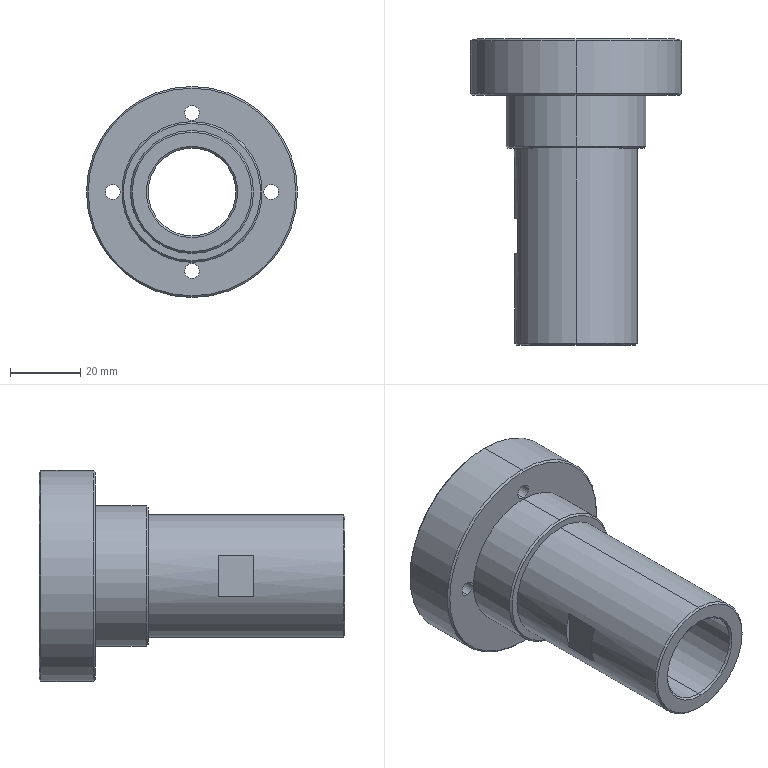Part | SolidWorks | features BaseBody 1 | 1 solid | 33 faces | box 60 x 87 x 60 mm | volume 74210 mm3 | cylinder 16 | cone 10 | plane 7 | commonest cylinder face diameters 4.2 x8 25 x2 35 x2 40 x2 60 x2
STEP:
#1=CARTESIAN_POINT('',(0.,-70.5,12.5));
#2=VERTEX_POINT('',#1);
#3=CARTESIAN_POINT('',(0.,-71.,13.));
#4=VERTEX_POINT('',#3);
#5=CARTESIAN_POINT('',(0.,-71.,13.));
#6=DIRECTION('',(0.,-0.7071,0.7071));
#7=VECTOR('',#6,1000.);
#8=LINE('',#5,#7);
#9=EDGE_CURVE('',#2,#4,#8,.T.);
#10=ORIENTED_EDGE('',*,*,#9,.F.);
#11=CARTESIAN_POINT('',(0.,-70.5,-12.5));
#12=VERTEX_POINT('',#11);
#13=CARTESIAN_POINT('',(0.,-70.5,0.));
#14=DIRECTION('',(0.,-1.,0.));
#15=DIRECTION('',(0.,0.,-1.));
#16=AXIS2_PLACEMENT_3D('',#13,#14,#15);
#17=CIRCLE('',#16,12.5);
#18=EDGE_CURVE('',#12,#2,#17,.T.);
#19=ORIENTED_EDGE('',*,*,#18,.F.);
#20=CARTESIAN_POINT('',(0.,-71.,-13.));
#21=VERTEX_POINT('',#20);
#22=CARTESIAN_POINT('',(0.,-71.,-13.));
#23=DIRECTION('',(0.,-0.7071,-0.7071));
#24=VECTOR('',#23,1000.);
#25=LINE('',#22,#24);
#26=EDGE_CURVE('',#12,#21,#25,.T.);
#27=ORIENTED_EDGE('',*,*,#26,.T.);
#28=CARTESIAN_POINT('',(0.,-71.,0.));
#29=DIRECTION('',(0.,1.,0.));
#30=DIRECTION('',(0.,0.,-1.));
#31=AXIS2_PLACEMENT_3D('',#28,#29,#30);
#32=CIRCLE('',#31,13.);
#33=EDGE_CURVE('',#4,#21,#32,.T.);
#34=ORIENTED_EDGE('',*,*,#33,.F.);
#35=EDGE_LOOP('',(#10,#19,#27,#34));
#36=FACE_OUTER_BOUND('',#35,.T.);
#37=CARTESIAN_POINT('',(0.,-71.,0.));
#38=DIRECTION('',(0.,-1.,0.));
#39=DIRECTION('',(0.,0.,-1.));
#40=AXIS2_PLACEMENT_3D('',#37,#38,#39);
#41=CONICAL_SURFACE('',#40,13.,0.7854);
#42=ADVANCED_FACE('',(#36),#41,.F.);
#43=CARTESIAN_POINT('',(-16.5,-45.,-5.831));
#44=VERTEX_POINT('',#43);
#45=CARTESIAN_POINT('',(-16.5,-45.,5.831));
#46=VERTEX_POINT('',#45);
#47=CARTESIAN_POINT('',(-16.5,-45.,-15.));
#48=DIRECTION('',(0.,0.,1.));
#49=VECTOR('',#48,1000.);
#50=LINE('',#47,#49);
#51=EDGE_CURVE('',#44,#46,#50,.T.);
#52=ORIENTED_EDGE('',*,*,#51,.F.);
#53=CARTESIAN_POINT('',(0.,-45.,0.));
#54=DIRECTION('',(0.,-1.,0.));
#55=DIRECTION('',(0.,0.,-1.));
#56=AXIS2_PLACEMENT_3D('',#53,#54,#55);
#57=CIRCLE('',#56,17.5);
#58=EDGE_CURVE('',#46,#44,#57,.T.);
#59=ORIENTED_EDGE('',*,*,#58,.F.);
#60=EDGE_LOOP('',(#52,#59));
#61=FACE_OUTER_BOUND('',#60,.T.);
#62=CARTESIAN_POINT('',(-17.5,-45.,-15.));
#63=DIRECTION('',(0.,-1.,0.));
#64=DIRECTION('',(0.,0.,-1.));
#65=AXIS2_PLACEMENT_3D('',#62,#63,#64);
#66=PLANE('',#65);
#67=ADVANCED_FACE('',(#61),#66,.F.);
#68=ORIENTED_EDGE('',*,*,#51,.T.);
#69=CARTESIAN_POINT('',(-16.5,-35.,5.831));
#70=VERTEX_POINT('',#69);
#71=CARTESIAN_POINT('',(-16.5,-71.,5.831));
#72=DIRECTION('',(0.,-1.,0.));
#73=VECTOR('',#72,1000.);
#74=LINE('',#71,#73);
#75=EDGE_CURVE('',#70,#46,#74,.T.);
#76=ORIENTED_EDGE('',*,*,#75,.F.);
#77=CARTESIAN_POINT('',(-16.5,-35.,-5.831));
#78=VERTEX_POINT('',#77);
#79=CARTESIAN_POINT('',(-16.5,-35.,-15.));
#80=DIRECTION('',(0.,0.,1.));
#81=VECTOR('',#80,1000.);
#82=LINE('',#79,#81);
#83=EDGE_CURVE('',#78,#70,#82,.T.);
#84=ORIENTED_EDGE('',*,*,#83,.F.);
#85=CARTESIAN_POINT('',(-16.5,-71.,-5.831));
#86=DIRECTION('',(0.,1.,0.));
#87=VECTOR('',#86,1000.);
#88=LINE('',#85,#87);
#89=EDGE_CURVE('',#44,#78,#88,.T.);
#90=ORIENTED_EDGE('',*,*,#89,.F.);
#91=EDGE_LOOP('',(#68,#76,#84,#90));
#92=FACE_OUTER_BOUND('',#91,.T.);
#93=CARTESIAN_POINT('',(-16.5,-45.,-15.));
#94=DIRECTION('',(1.,0.,0.));
#95=DIRECTION('',(0.,1.,0.));
#96=AXIS2_PLACEMENT_3D('',#93,#94,#95);
#97=PLANE('',#96);
#98=ADVANCED_FACE('',(#92),#97,.F.);
#99=ORIENTED_EDGE('',*,*,#83,.T.);
#100=CARTESIAN_POINT('',(0.,-35.,0.));
#101=DIRECTION('',(0.,1.,0.));
#102=DIRECTION('',(0.,0.,1.));
#103=AXIS2_PLACEMENT_3D('',#100,#101,#102);
#104=CIRCLE('',#103,17.5);
#105=EDGE_CURVE('',#78,#70,#104,.T.);
#106=ORIENTED_EDGE('',*,*,#105,.F.);
#107=EDGE_LOOP('',(#99,#106));
#108=FACE_OUTER_BOUND('',#107,.T.);
#109=CARTESIAN_POINT('',(-17.5,-35.,-15.));
#110=DIRECTION('',(0.,1.,0.));
#111=DIRECTION('',(1.,0.,0.));
#112=AXIS2_PLACEMENT_3D('',#109,#110,#111);
#113=PLANE('',#112);
#114=ADVANCED_FACE('',(#108),#113,.F.);
#115=CARTESIAN_POINT('',(0.,16.,-12.5));
#116=VERTEX_POINT('',#115);
#117=CARTESIAN_POINT('',(0.,-106.355,-12.5));
#118=DIRECTION('',(0.,1.,0.));
#119=VECTOR('',#118,1000.);
#120=LINE('',#117,#119);
#121=EDGE_CURVE('',#12,#116,#120,.T.);
#122=ORIENTED_EDGE('',*,*,#121,.F.);
#123=ORIENTED_EDGE('',*,*,#18,.T.);
#124=CARTESIAN_POINT('',(0.,16.,12.5));
#125=VERTEX_POINT('',#124);
#126=CARTESIAN_POINT('',(0.,-106.355,12.5));
#127=DIRECTION('',(0.,1.,0.));
#128=VECTOR('',#127,1000.);
#129=LINE('',#126,#128);
#130=EDGE_CURVE('',#2,#125,#129,.T.);
#131=ORIENTED_EDGE('',*,*,#130,.T.);
#132=CARTESIAN_POINT('',(0.,16.,0.));
#133=DIRECTION('',(0.,1.,0.));
#134=DIRECTION('',(0.,0.,1.));
#135=AXIS2_PLACEMENT_3D('',#132,#133,#134);
#136=CIRCLE('',#135,12.5);
#137=EDGE_CURVE('',#125,#116,#136,.T.);
#138=ORIENTED_EDGE('',*,*,#137,.T.);
#139=EDGE_LOOP('',(#122,#123,#131,#138));
#140=FACE_OUTER_BOUND('',#139,.T.);
#141=CARTESIAN_POINT('',(0.,-106.355,0.));
#142=DIRECTION('',(0.,1.,0.));
#143=DIRECTION('',(0.,0.,1.));
#144=AXIS2_PLACEMENT_3D('',#141,#142,#143);
#145=CYLINDRICAL_SURFACE('',#144,12.5);
#146=ADVANCED_FACE('',(#140),#145,.F.);
#147=CARTESIAN_POINT('',(0.,0.,20.4));
#148=VERTEX_POINT('',#147);
#149=CARTESIAN_POINT('',(0.,16.,20.4));
#150=VERTEX_POINT('',#149);
#151=CARTESIAN_POINT('',(0.,16.,20.4));
#152=DIRECTION('',(0.,1.,0.));
#153=VECTOR('',#152,1000.);
#154=LINE('',#151,#153);
#155=EDGE_CURVE('',#148,#150,#154,.T.);
#156=ORIENTED_EDGE('',*,*,#155,.F.);
#157=CARTESIAN_POINT('',(0.,0.,24.6));
#158=VERTEX_POINT('',#157);
#159=CARTESIAN_POINT('',(0.,0.,22.5));
#160=DIRECTION('',(0.,1.,0.));
#161=DIRECTION('',(0.,0.,1.));
#162=AXIS2_PLACEMENT_3D('',#159,#160,#161);
#163=CIRCLE('',#162,2.1);
#164=EDGE_CURVE('',#158,#148,#163,.T.);
#165=ORIENTED_EDGE('',*,*,#164,.F.);
#166=CARTESIAN_POINT('',(0.,16.,24.6));
#167=VERTEX_POINT('',#166);
#168=CARTESIAN_POINT('',(0.,16.,24.6));
#169=DIRECTION('',(0.,1.,0.));
#170=VECTOR('',#169,1000.);
#171=LINE('',#168,#170);
#172=EDGE_CURVE('',#158,#167,#171,.T.);
#173=ORIENTED_EDGE('',*,*,#172,.T.);
#174=CARTESIAN_POINT('',(0.,16.,22.5));
#175=DIRECTION('',(0.,1.,0.));
#176=DIRECTION('',(0.,0.,1.));
#177=AXIS2_PLACEMENT_3D('',#174,#175,#176);
#178=CIRCLE('',#177,2.1);
#179=EDGE_CURVE('',#167,#150,#178,.T.);
#180=ORIENTED_EDGE('',*,*,#179,.T.);
#181=EDGE_LOOP('',(#156,#165,#173,#180));
#182=FACE_OUTER_BOUND('',#181,.T.);
#183=CARTESIAN_POINT('',(0.,16.,22.5));
#184=DIRECTION('',(0.,1.,0.));
#185=DIRECTION('',(0.,0.,1.));
#186=AXIS2_PLACEMENT_3D('',#183,#184,#185);
#187=CYLINDRICAL_SURFACE('',#186,2.1);
#188=ADVANCED_FACE('',(#182),#187,.F.);
#189=CARTESIAN_POINT('',(0.,0.,-24.6));
#190=VERTEX_POINT('',#189);
#191=CARTESIAN_POINT('',(0.,16.,-24.6));
#192=VERTEX_POINT('',#191);
#193=CARTESIAN_POINT('',(0.,16.,-24.6));
#194=DIRECTION('',(0.,1.,0.));
#195=VECTOR('',#194,1000.);
#196=LINE('',#193,#195);
#197=EDGE_CURVE('',#190,#192,#196,.T.);
#198=ORIENTED_EDGE('',*,*,#197,.F.);
#199=CARTESIAN_POINT('',(0.,0.,-20.4));
#200=VERTEX_POINT('',#199);
#201=CARTESIAN_POINT('',(0.,0.,-22.5));
#202=DIRECTION('',(0.,1.,0.));
#203=DIRECTION('',(0.,0.,1.));
#204=AXIS2_PLACEMENT_3D('',#201,#202,#203);
#205=CIRCLE('',#204,2.1);
#206=EDGE_CURVE('',#200,#190,#205,.T.);
#207=ORIENTED_EDGE('',*,*,#206,.F.);
#208=CARTESIAN_POINT('',(0.,16.,-20.4));
#209=VERTEX_POINT('',#208);
#210=CARTESIAN_POINT('',(0.,16.,-20.4));
#211=DIRECTION('',(0.,1.,0.));
#212=VECTOR('',#211,1000.);
#213=LINE('',#210,#212);
#214=EDGE_CURVE('',#200,#209,#213,.T.);
#215=ORIENTED_EDGE('',*,*,#214,.T.);
#216=CARTESIAN_POINT('',(0.,16.,-22.5));
#217=DIRECTION('',(0.,1.,0.));
#218=DIRECTION('',(0.,0.,1.));
#219=AXIS2_PLACEMENT_3D('',#216,#217,#218);
#220=CIRCLE('',#219,2.1);
#221=EDGE_CURVE('',#209,#192,#220,.T.);
#222=ORIENTED_EDGE('',*,*,#221,.T.);
#223=EDGE_LOOP('',(#198,#207,#215,#222));
#224=FACE_OUTER_BOUND('',#223,.T.);
#225=CARTESIAN_POINT('',(0.,16.,-22.5));
#226=DIRECTION('',(0.,1.,0.));
#227=DIRECTION('',(0.,0.,1.));
#228=AXIS2_PLACEMENT_3D('',#225,#226,#227);
#229=CYLINDRICAL_SURFACE('',#228,2.1);
#230=ADVANCED_FACE('',(#224),#229,.F.);
#231=CARTESIAN_POINT('',(22.5,0.,-2.1));
#232=VERTEX_POINT('',#231);
#233=CARTESIAN_POINT('',(22.5,16.,-2.1));
#234=VERTEX_POINT('',#233);
#235=CARTESIAN_POINT('',(22.5,16.,-2.1));
#236=DIRECTION('',(0.,1.,0.));
#237=VECTOR('',#236,1000.);
#238=LINE('',#235,#237);
#239=EDGE_CURVE('',#232,#234,#238,.T.);
#240=ORIENTED_EDGE('',*,*,#239,.F.);
#241=CARTESIAN_POINT('',(22.5,0.,2.1));
#242=VERTEX_POINT('',#241);
#243=CARTESIAN_POINT('',(22.5,0.,0.));
#244=DIRECTION('',(0.,1.,0.));
#245=DIRECTION('',(0.,0.,1.));
#246=AXIS2_PLACEMENT_3D('',#243,#244,#245);
#247=CIRCLE('',#246,2.1);
#248=EDGE_CURVE('',#242,#232,#247,.T.);
#249=ORIENTED_EDGE('',*,*,#248,.F.);
#250=CARTESIAN_POINT('',(22.5,16.,2.1));
#251=VERTEX_POINT('',#250);
#252=CARTESIAN_POINT('',(22.5,16.,2.1));
#253=DIRECTION('',(0.,1.,0.));
#254=VECTOR('',#253,1000.);
#255=LINE('',#252,#254);
#256=EDGE_CURVE('',#242,#251,#255,.T.);
#257=ORIENTED_EDGE('',*,*,#256,.T.);
#258=CARTESIAN_POINT('',(22.5,16.,0.));
#259=DIRECTION('',(0.,1.,0.));
#260=DIRECTION('',(0.,0.,1.));
#261=AXIS2_PLACEMENT_3D('',#258,#259,#260);
#262=CIRCLE('',#261,2.1);
#263=EDGE_CURVE('',#251,#234,#262,.T.);
#264=ORIENTED_EDGE('',*,*,#263,.T.);
#265=EDGE_LOOP('',(#240,#249,#257,#264));
#266=FACE_OUTER_BOUND('',#265,.T.);
#267=CARTESIAN_POINT('',(22.5,16.,0.));
#268=DIRECTION('',(0.,1.,0.));
#269=DIRECTION('',(0.,0.,1.));
#270=AXIS2_PLACEMENT_3D('',#267,#268,#269);
#271=CYLINDRICAL_SURFACE('',#270,2.1);
#272=ADVANCED_FACE('',(#266),#271,.F.);
#273=CARTESIAN_POINT('',(-22.5,0.,-2.1));
#274=VERTEX_POINT('',#273);
#275=CARTESIAN_POINT('',(-22.5,16.,-2.1));
#276=VERTEX_POINT('',#275);
#277=CARTESIAN_POINT('',(-22.5,16.,-2.1));
#278=DIRECTION('',(0.,1.,0.));
#279=VECTOR('',#278,1000.);
#280=LINE('',#277,#279);
#281=EDGE_CURVE('',#274,#276,#280,.T.);
#282=ORIENTED_EDGE('',*,*,#281,.F.);
#283=CARTESIAN_POINT('',(-22.5,0.,2.1));
#284=VERTEX_POINT('',#283);
#285=CARTESIAN_POINT('',(-22.5,0.,0.));
#286=DIRECTION('',(0.,1.,0.));
#287=DIRECTION('',(0.,0.,1.));
#288=AXIS2_PLACEMENT_3D('',#285,#286,#287);
#289=CIRCLE('',#288,2.1);
#290=EDGE_CURVE('',#284,#274,#289,.T.);
#291=ORIENTED_EDGE('',*,*,#290,.F.);
#292=CARTESIAN_POINT('',(-22.5,16.,2.1));
#293=VERTEX_POINT('',#292);
#294=CARTESIAN_POINT('',(-22.5,16.,2.1));
#295=DIRECTION('',(0.,1.,0.));
#296=VECTOR('',#295,1000.);
#297=LINE('',#294,#296);
#298=EDGE_CURVE('',#284,#293,#297,.T.);
#299=ORIENTED_EDGE('',*,*,#298,.T.);
#300=CARTESIAN_POINT('',(-22.5,16.,0.));
#301=DIRECTION('',(0.,1.,0.));
#302=DIRECTION('',(0.,0.,1.));
#303=AXIS2_PLACEMENT_3D('',#300,#301,#302);
#304=CIRCLE('',#303,2.1);
#305=EDGE_CURVE('',#293,#276,#304,.T.);
#306=ORIENTED_EDGE('',*,*,#305,.T.);
#307=EDGE_LOOP('',(#282,#291,#299,#306));
#308=FACE_OUTER_BOUND('',#307,.T.);
#309=CARTESIAN_POINT('',(-22.5,16.,0.));
#310=DIRECTION('',(0.,1.,0.));
#311=DIRECTION('',(0.,0.,1.));
#312=AXIS2_PLACEMENT_3D('',#309,#310,#311);
#313=CYLINDRICAL_SURFACE('',#312,2.1);
#314=ADVANCED_FACE('',(#308),#313,.F.);
#315=CARTESIAN_POINT('',(0.,16.,29.5));
#316=VERTEX_POINT('',#315);
#317=CARTESIAN_POINT('',(0.,15.5,30.));
#318=VERTEX_POINT('',#317);
#319=CARTESIAN_POINT('',(0.,16.,29.5));
#320=DIRECTION('',(0.,-0.7071,0.7071));
#321=VECTOR('',#320,1000.);
#322=LINE('',#319,#321);
#323=EDGE_CURVE('',#316,#318,#322,.T.);
#324=ORIENTED_EDGE('',*,*,#323,.F.);
#325=CARTESIAN_POINT('',(0.,16.,-29.5));
#326=VERTEX_POINT('',#325);
#327=CARTESIAN_POINT('',(0.,16.,0.));
#328=DIRECTION('',(0.,1.,0.));
#329=DIRECTION('',(0.,0.,1.));
#330=AXIS2_PLACEMENT_3D('',#327,#328,#329);
#331=CIRCLE('',#330,29.5);
#332=EDGE_CURVE('',#326,#316,#331,.T.);
#333=ORIENTED_EDGE('',*,*,#332,.F.);
#334=CARTESIAN_POINT('',(0.,15.5,-30.));
#335=VERTEX_POINT('',#334);
#336=CARTESIAN_POINT('',(0.,16.,-29.5));
#337=DIRECTION('',(0.,-0.7071,-0.7071));
#338=VECTOR('',#337,1000.);
#339=LINE('',#336,#338);
#340=EDGE_CURVE('',#326,#335,#339,.T.);
#341=ORIENTED_EDGE('',*,*,#340,.T.);
#342=CARTESIAN_POINT('',(0.,15.5,0.));
#343=DIRECTION('',(0.,-1.,0.));
#344=DIRECTION('',(0.,0.,1.));
#345=AXIS2_PLACEMENT_3D('',#342,#343,#344);
#346=CIRCLE('',#345,30.);
#347=EDGE_CURVE('',#318,#335,#346,.T.);
#348=ORIENTED_EDGE('',*,*,#347,.F.);
#349=EDGE_LOOP('',(#324,#333,#341,#348));
#350=FACE_OUTER_BOUND('',#349,.T.);
#351=CARTESIAN_POINT('',(0.,16.,0.));
#352=DIRECTION('',(0.,-1.,0.));
#353=DIRECTION('',(0.,0.,-1.));
#354=AXIS2_PLACEMENT_3D('',#351,#352,#353);
#355=CONICAL_SURFACE('',#354,29.5,0.7854);
#356=ADVANCED_FACE('',(#350),#355,.T.);
#357=CARTESIAN_POINT('',(0.,0.,-29.5));
#358=VERTEX_POINT('',#357);
#359=CARTESIAN_POINT('',(0.,0.5,-30.));
#360=VERTEX_POINT('',#359);
#361=CARTESIAN_POINT('',(0.,0.5,-30.));
#362=DIRECTION('',(0.,0.7071,-0.7071));
#363=VECTOR('',#362,1000.);
#364=LINE('',#361,#363);
#365=EDGE_CURVE('',#358,#360,#364,.T.);
#366=ORIENTED_EDGE('',*,*,#365,.F.);
#367=CARTESIAN_POINT('',(0.,0.,29.5));
#368=VERTEX_POINT('',#367);
#369=CARTESIAN_POINT('',(0.,0.,0.));
#370=DIRECTION('',(0.,-1.,0.));
#371=DIRECTION('',(0.,0.,1.));
#372=AXIS2_PLACEMENT_3D('',#369,#370,#371);
#373=CIRCLE('',#372,29.5);
#374=EDGE_CURVE('',#368,#358,#373,.T.);
#375=ORIENTED_EDGE('',*,*,#374,.F.);
#376=CARTESIAN_POINT('',(0.,0.5,30.));
#377=VERTEX_POINT('',#376);
#378=CARTESIAN_POINT('',(0.,0.5,30.));
#379=DIRECTION('',(0.,0.7071,0.7071));
#380=VECTOR('',#379,1000.);
#381=LINE('',#378,#380);
#382=EDGE_CURVE('',#368,#377,#381,.T.);
#383=ORIENTED_EDGE('',*,*,#382,.T.);
#384=CARTESIAN_POINT('',(0.,0.5,0.));
#385=DIRECTION('',(0.,1.,0.));
#386=DIRECTION('',(0.,0.,1.));
#387=AXIS2_PLACEMENT_3D('',#384,#385,#386);
#388=CIRCLE('',#387,30.);
#389=EDGE_CURVE('',#360,#377,#388,.T.);
#390=ORIENTED_EDGE('',*,*,#389,.F.);
#391=EDGE_LOOP('',(#366,#375,#383,#390));
#392=FACE_OUTER_BOUND('',#391,.T.);
#393=CARTESIAN_POINT('',(0.,0.5,0.));
#394=DIRECTION('',(0.,1.,0.));
#395=DIRECTION('',(0.,0.,1.));
#396=AXIS2_PLACEMENT_3D('',#393,#394,#395);
#397=CONICAL_SURFACE('',#396,30.,0.7854);
#398=ADVANCED_FACE('',(#392),#397,.T.);
#399=CARTESIAN_POINT('',(0.,-15.,-19.5));
#400=VERTEX_POINT('',#399);
#401=CARTESIAN_POINT('',(0.,-14.5,-20.));
#402=VERTEX_POINT('',#401);
#403=CARTESIAN_POINT('',(0.,-15.,-19.5));
#404=DIRECTION('',(0.,0.7071,-0.7071));
#405=VECTOR('',#404,1000.);
#406=LINE('',#403,#405);
#407=EDGE_CURVE('',#400,#402,#406,.T.);
#408=ORIENTED_EDGE('',*,*,#407,.F.);
#409=CARTESIAN_POINT('',(0.,-15.,19.5));
#410=VERTEX_POINT('',#409);
#411=CARTESIAN_POINT('',(0.,-15.,0.));
#412=DIRECTION('',(0.,-1.,0.));
#413=DIRECTION('',(0.,0.,-1.));
#414=AXIS2_PLACEMENT_3D('',#411,#412,#413);
#415=CIRCLE('',#414,19.5);
#416=EDGE_CURVE('',#410,#400,#415,.T.);
#417=ORIENTED_EDGE('',*,*,#416,.F.);
#418=CARTESIAN_POINT('',(0.,-14.5,20.));
#419=VERTEX_POINT('',#418);
#420=CARTESIAN_POINT('',(0.,-15.,19.5));
#421=DIRECTION('',(0.,0.7071,0.7071));
#422=VECTOR('',#421,1000.);
#423=LINE('',#420,#422);
#424=EDGE_CURVE('',#410,#419,#423,.T.);
#425=ORIENTED_EDGE('',*,*,#424,.T.);
#426=CARTESIAN_POINT('',(0.,-14.5,0.));
#427=DIRECTION('',(0.,1.,0.));
#428=DIRECTION('',(0.,0.,-1.));
#429=AXIS2_PLACEMENT_3D('',#426,#427,#428);
#430=CIRCLE('',#429,20.);
#431=EDGE_CURVE('',#402,#419,#430,.T.);
#432=ORIENTED_EDGE('',*,*,#431,.F.);
#433=EDGE_LOOP('',(#408,#417,#425,#432));
#434=FACE_OUTER_BOUND('',#433,.T.);
#435=CARTESIAN_POINT('',(0.,-15.,0.));
#436=DIRECTION('',(0.,1.,0.));
#437=DIRECTION('',(0.,0.,1.));
#438=AXIS2_PLACEMENT_3D('',#435,#436,#437);
#439=CONICAL_SURFACE('',#438,19.5,0.7854);
#440=ADVANCED_FACE('',(#434),#439,.T.);
#441=CARTESIAN_POINT('',(0.,-71.,-17.));
#442=VERTEX_POINT('',#441);
#443=CARTESIAN_POINT('',(0.,-70.5,-17.5));
#444=VERTEX_POINT('',#443);
#445=CARTESIAN_POINT('',(0.,-71.,-17.));
#446=DIRECTION('',(0.,0.7071,-0.7071));
#447=VECTOR('',#446,1000.);
#448=LINE('',#445,#447);
#449=EDGE_CURVE('',#442,#444,#448,.T.);
#450=ORIENTED_EDGE('',*,*,#449,.F.);
#451=CARTESIAN_POINT('',(0.,-71.,17.));
#452=VERTEX_POINT('',#451);
#453=CARTESIAN_POINT('',(0.,-71.,0.));
#454=DIRECTION('',(0.,-1.,0.));
#455=DIRECTION('',(0.,0.,-1.));
#456=AXIS2_PLACEMENT_3D('',#453,#454,#455);
#457=CIRCLE('',#456,17.);
#458=EDGE_CURVE('',#452,#442,#457,.T.);
#459=ORIENTED_EDGE('',*,*,#458,.F.);
#460=CARTESIAN_POINT('',(0.,-70.5,17.5));
#461=VERTEX_POINT('',#460);
#462=CARTESIAN_POINT('',(0.,-71.,17.));
#463=DIRECTION('',(0.,0.7071,0.7071));
#464=VECTOR('',#463,1000.);
#465=LINE('',#462,#464);
#466=EDGE_CURVE('',#452,#461,#465,.T.);
#467=ORIENTED_EDGE('',*,*,#466,.T.);
#468=CARTESIAN_POINT('',(0.,-70.5,0.));
#469=DIRECTION('',(0.,1.,0.));
#470=DIRECTION('',(0.,0.,-1.));
#471=AXIS2_PLACEMENT_3D('',#468,#469,#470);
#472=CIRCLE('',#471,17.5);
#473=EDGE_CURVE('',#444,#461,#472,.T.);
#474=ORIENTED_EDGE('',*,*,#473,.F.);
#475=EDGE_LOOP('',(#450,#459,#467,#474));
#476=FACE_OUTER_BOUND('',#475,.T.);
#477=CARTESIAN_POINT('',(0.,-71.,0.));
#478=DIRECTION('',(0.,1.,0.));
#479=DIRECTION('',(0.,0.,1.));
#480=AXIS2_PLACEMENT_3D('',#477,#478,#479);
#481=CONICAL_SURFACE('',#480,17.,0.7854);
#482=ADVANCED_FACE('',(#476),#481,.T.);
#483=CARTESIAN_POINT('',(0.,-71.,0.));
#484=DIRECTION('',(0.,1.,0.));
#485=DIRECTION('',(0.,0.,-1.));
#486=AXIS2_PLACEMENT_3D('',#483,#484,#485);
#487=CIRCLE('',#486,13.);
#488=EDGE_CURVE('',#21,#4,#487,.T.);
#489=ORIENTED_EDGE('',*,*,#488,.T.);
#490=ORIENTED_EDGE('',*,*,#33,.T.);
#491=EDGE_LOOP('',(#489,#490));
#492=FACE_BOUND('',#491,.T.);
#493=ORIENTED_EDGE('',*,*,#458,.T.);
#494=CARTESIAN_POINT('',(0.,-71.,0.));
#495=DIRECTION('',(0.,-1.,0.));
#496=DIRECTION('',(0.,0.,-1.));
#497=AXIS2_PLACEMENT_3D('',#494,#495,#496);
#498=CIRCLE('',#497,17.);
#499=EDGE_CURVE('',#442,#452,#498,.T.);
#500=ORIENTED_EDGE('',*,*,#499,.T.);
#501=EDGE_LOOP('',(#493,#500));
#502=FACE_OUTER_BOUND('',#501,.T.);
#503=CARTESIAN_POINT('',(0.,-71.,0.));
#504=DIRECTION('',(0.,-1.,0.));
#505=DIRECTION('',(0.,0.,-1.));
#506=AXIS2_PLACEMENT_3D('',#503,#504,#505);
#507=PLANE('',#506);
#508=ADVANCED_FACE('',(#492,#502),#507,.T.);
#509=ORIENTED_EDGE('',*,*,#89,.T.);
#510=ORIENTED_EDGE('',*,*,#105,.T.);
#511=ORIENTED_EDGE('',*,*,#75,.T.);
#512=ORIENTED_EDGE('',*,*,#58,.T.);
#513=EDGE_LOOP('',(#509,#510,#511,#512));
#514=FACE_BOUND('',#513,.T.);
#515=CARTESIAN_POINT('',(0.,-15.,-17.5));
#516=VERTEX_POINT('',#515);
#517=CARTESIAN_POINT('',(0.,-71.,-17.5));
#518=DIRECTION('',(0.,1.,0.));
#519=VECTOR('',#518,1000.);
#520=LINE('',#517,#519);
#521=EDGE_CURVE('',#444,#516,#520,.T.);
#522=ORIENTED_EDGE('',*,*,#521,.F.);
#523=ORIENTED_EDGE('',*,*,#473,.T.);
#524=CARTESIAN_POINT('',(0.,-15.,17.5));
#525=VERTEX_POINT('',#524);
#526=CARTESIAN_POINT('',(0.,-71.,17.5));
#527=DIRECTION('',(0.,1.,0.));
#528=VECTOR('',#527,1000.);
#529=LINE('',#526,#528);
#530=EDGE_CURVE('',#461,#525,#529,.T.);
#531=ORIENTED_EDGE('',*,*,#530,.T.);
#532=CARTESIAN_POINT('',(0.,-15.,0.));
#533=DIRECTION('',(0.,-1.,0.));
#534=DIRECTION('',(0.,0.,-1.));
#535=AXIS2_PLACEMENT_3D('',#532,#533,#534);
#536=CIRCLE('',#535,17.5);
#537=EDGE_CURVE('',#525,#516,#536,.T.);
#538=ORIENTED_EDGE('',*,*,#537,.T.);
#539=EDGE_LOOP('',(#522,#523,#531,#538));
#540=FACE_OUTER_BOUND('',#539,.T.);
#541=CARTESIAN_POINT('',(0.,-71.,0.));
#542=DIRECTION('',(0.,1.,0.));
#543=DIRECTION('',(0.,0.,1.));
#544=AXIS2_PLACEMENT_3D('',#541,#542,#543);
#545=CYLINDRICAL_SURFACE('',#544,17.5);
#546=ADVANCED_FACE('',(#514,#540),#545,.T.);
#547=ORIENTED_EDGE('',*,*,#537,.F.);
#548=CARTESIAN_POINT('',(0.,-15.,0.));
#549=DIRECTION('',(0.,-1.,0.));
#550=DIRECTION('',(0.,0.,-1.));
#551=AXIS2_PLACEMENT_3D('',#548,#549,#550);
#552=CIRCLE('',#551,17.5);
#553=EDGE_CURVE('',#516,#525,#552,.T.);
#554=ORIENTED_EDGE('',*,*,#553,.F.);
#555=EDGE_LOOP('',(#547,#554));
#556=FACE_BOUND('',#555,.T.);
#557=ORIENTED_EDGE('',*,*,#416,.T.);
#558=CARTESIAN_POINT('',(0.,-15.,0.));
#559=DIRECTION('',(0.,-1.,0.));
#560=DIRECTION('',(0.,0.,-1.));
#561=AXIS2_PLACEMENT_3D('',#558,#559,#560);
#562=CIRCLE('',#561,19.5);
#563=EDGE_CURVE('',#400,#410,#562,.T.);
#564=ORIENTED_EDGE('',*,*,#563,.T.);
#565=EDGE_LOOP('',(#557,#564));
#566=FACE_OUTER_BOUND('',#565,.T.);
#567=CARTESIAN_POINT('',(0.,-15.,0.));
#568=DIRECTION('',(0.,-1.,0.));
#569=DIRECTION('',(0.,0.,-1.));
#570=AXIS2_PLACEMENT_3D('',#567,#568,#569);
#571=PLANE('',#570);
#572=ADVANCED_FACE('',(#556,#566),#571,.T.);
#573=CARTESIAN_POINT('',(0.,0.,-20.));
#574=VERTEX_POINT('',#573);
#575=CARTESIAN_POINT('',(0.,-15.,-20.));
#576=DIRECTION('',(0.,1.,0.));
#577=VECTOR('',#576,1000.);
#578=LINE('',#575,#577);
#579=EDGE_CURVE('',#402,#574,#578,.T.);
#580=ORIENTED_EDGE('',*,*,#579,.F.);
#581=ORIENTED_EDGE('',*,*,#431,.T.);
#582=CARTESIAN_POINT('',(0.,0.,20.));
#583=VERTEX_POINT('',#582);
#584=CARTESIAN_POINT('',(0.,-15.,20.));
#585=DIRECTION('',(0.,1.,0.));
#586=VECTOR('',#585,1000.);
#587=LINE('',#584,#586);
#588=EDGE_CURVE('',#419,#583,#587,.T.);
#589=ORIENTED_EDGE('',*,*,#588,.T.);
#590=CARTESIAN_POINT('',(0.,0.,0.));
#591=DIRECTION('',(0.,-1.,0.));
#592=DIRECTION('',(0.,0.,-1.));
#593=AXIS2_PLACEMENT_3D('',#590,#591,#592);
#594=CIRCLE('',#593,20.);
#595=EDGE_CURVE('',#583,#574,#594,.T.);
#596=ORIENTED_EDGE('',*,*,#595,.T.);
#597=EDGE_LOOP('',(#580,#581,#589,#596));
#598=FACE_OUTER_BOUND('',#597,.T.);
#599=CARTESIAN_POINT('',(0.,-15.,0.));
#600=DIRECTION('',(0.,1.,0.));
#601=DIRECTION('',(0.,0.,1.));
#602=AXIS2_PLACEMENT_3D('',#599,#600,#601);
#603=CYLINDRICAL_SURFACE('',#602,20.);
#604=ADVANCED_FACE('',(#598),#603,.T.);
#605=ORIENTED_EDGE('',*,*,#595,.F.);
#606=CARTESIAN_POINT('',(0.,0.,0.));
#607=DIRECTION('',(0.,-1.,0.));
#608=DIRECTION('',(0.,0.,-1.));
#609=AXIS2_PLACEMENT_3D('',#606,#607,#608);
#610=CIRCLE('',#609,20.);
#611=EDGE_CURVE('',#574,#583,#610,.T.);
#612=ORIENTED_EDGE('',*,*,#611,.F.);
#613=EDGE_LOOP('',(#605,#612));
#614=FACE_BOUND('',#613,.T.);
#615=ORIENTED_EDGE('',*,*,#290,.T.);
#616=CARTESIAN_POINT('',(-22.5,0.,0.));
#617=DIRECTION('',(0.,1.,0.));
#618=DIRECTION('',(0.,0.,1.));
#619=AXIS2_PLACEMENT_3D('',#616,#617,#618);
#620=CIRCLE('',#619,2.1);
#621=EDGE_CURVE('',#274,#284,#620,.T.);
#622=ORIENTED_EDGE('',*,*,#621,.T.);
#623=EDGE_LOOP('',(#615,#622));
#624=FACE_BOUND('',#623,.T.);
#625=ORIENTED_EDGE('',*,*,#248,.T.);
#626=CARTESIAN_POINT('',(22.5,0.,0.));
#627=DIRECTION('',(0.,1.,0.));
#628=DIRECTION('',(0.,0.,1.));
#629=AXIS2_PLACEMENT_3D('',#626,#627,#628);
#630=CIRCLE('',#629,2.1);
#631=EDGE_CURVE('',#232,#242,#630,.T.);
#632=ORIENTED_EDGE('',*,*,#631,.T.);
#633=EDGE_LOOP('',(#625,#632));
#634=FACE_BOUND('',#633,.T.);
#635=ORIENTED_EDGE('',*,*,#206,.T.);
#636=CARTESIAN_POINT('',(0.,0.,-22.5));
#637=DIRECTION('',(0.,1.,0.));
#638=DIRECTION('',(0.,0.,1.));
#639=AXIS2_PLACEMENT_3D('',#636,#637,#638);
#640=CIRCLE('',#639,2.1);
#641=EDGE_CURVE('',#190,#200,#640,.T.);
#642=ORIENTED_EDGE('',*,*,#641,.T.);
#643=EDGE_LOOP('',(#635,#642));
#644=FACE_BOUND('',#643,.T.);
#645=ORIENTED_EDGE('',*,*,#164,.T.);
#646=CARTESIAN_POINT('',(0.,0.,22.5));
#647=DIRECTION('',(0.,1.,0.));
#648=DIRECTION('',(0.,0.,1.));
#649=AXIS2_PLACEMENT_3D('',#646,#647,#648);
#650=CIRCLE('',#649,2.1);
#651=EDGE_CURVE('',#148,#158,#650,.T.);
#652=ORIENTED_EDGE('',*,*,#651,.T.);
#653=EDGE_LOOP('',(#645,#652));
#654=FACE_BOUND('',#653,.T.);
#655=ORIENTED_EDGE('',*,*,#374,.T.);
#656=CARTESIAN_POINT('',(0.,0.,0.));
#657=DIRECTION('',(0.,-1.,0.));
#658=DIRECTION('',(0.,0.,1.));
#659=AXIS2_PLACEMENT_3D('',#656,#657,#658);
#660=CIRCLE('',#659,29.5);
#661=EDGE_CURVE('',#358,#368,#660,.T.);
#662=ORIENTED_EDGE('',*,*,#661,.T.);
#663=EDGE_LOOP('',(#655,#662));
#664=FACE_OUTER_BOUND('',#663,.T.);
#665=CARTESIAN_POINT('',(0.,0.,0.));
#666=DIRECTION('',(0.,1.,0.));
#667=DIRECTION('',(1.,0.,0.));
#668=AXIS2_PLACEMENT_3D('',#665,#666,#667);
#669=PLANE('',#668);
#670=ADVANCED_FACE('',(#614,#624,#634,#644,#654,#664),#669,.F.);
#671=ORIENTED_EDGE('',*,*,#305,.F.);
#672=CARTESIAN_POINT('',(-22.5,16.,0.));
#673=DIRECTION('',(0.,1.,0.));
#674=DIRECTION('',(0.,0.,1.));
#675=AXIS2_PLACEMENT_3D('',#672,#673,#674);
#676=CIRCLE('',#675,2.1);
#677=EDGE_CURVE('',#276,#293,#676,.T.);
#678=ORIENTED_EDGE('',*,*,#677,.F.);
#679=EDGE_LOOP('',(#671,#678));
#680=FACE_BOUND('',#679,.T.);
#681=ORIENTED_EDGE('',*,*,#263,.F.);
#682=CARTESIAN_POINT('',(22.5,16.,0.));
#683=DIRECTION('',(0.,1.,0.));
#684=DIRECTION('',(0.,0.,1.));
#685=AXIS2_PLACEMENT_3D('',#682,#683,#684);
#686=CIRCLE('',#685,2.1);
#687=EDGE_CURVE('',#234,#251,#686,.T.);
#688=ORIENTED_EDGE('',*,*,#687,.F.);
#689=EDGE_LOOP('',(#681,#688));
#690=FACE_BOUND('',#689,.T.);
#691=ORIENTED_EDGE('',*,*,#221,.F.);
#692=CARTESIAN_POINT('',(0.,16.,-22.5));
#693=DIRECTION('',(0.,1.,0.));
#694=DIRECTION('',(0.,0.,1.));
#695=AXIS2_PLACEMENT_3D('',#692,#693,#694);
#696=CIRCLE('',#695,2.1);
#697=EDGE_CURVE('',#192,#209,#696,.T.);
#698=ORIENTED_EDGE('',*,*,#697,.F.);
#699=EDGE_LOOP('',(#691,#698));
#700=FACE_BOUND('',#699,.T.);
#701=ORIENTED_EDGE('',*,*,#179,.F.);
#702=CARTESIAN_POINT('',(0.,16.,22.5));
#703=DIRECTION('',(0.,1.,0.));
#704=DIRECTION('',(0.,0.,1.));
#705=AXIS2_PLACEMENT_3D('',#702,#703,#704);
#706=CIRCLE('',#705,2.1);
#707=EDGE_CURVE('',#150,#167,#706,.T.);
#708=ORIENTED_EDGE('',*,*,#707,.F.);
#709=EDGE_LOOP('',(#701,#708));
#710=FACE_BOUND('',#709,.T.);
#711=ORIENTED_EDGE('',*,*,#137,.F.);
#712=CARTESIAN_POINT('',(0.,16.,0.));
#713=DIRECTION('',(0.,1.,0.));
#714=DIRECTION('',(0.,0.,1.));
#715=AXIS2_PLACEMENT_3D('',#712,#713,#714);
#716=CIRCLE('',#715,12.5);
#717=EDGE_CURVE('',#116,#125,#716,.T.);
#718=ORIENTED_EDGE('',*,*,#717,.F.);
#719=EDGE_LOOP('',(#711,#718));
#720=FACE_BOUND('',#719,.T.);
#721=ORIENTED_EDGE('',*,*,#332,.T.);
#722=CARTESIAN_POINT('',(0.,16.,0.));
#723=DIRECTION('',(0.,1.,0.));
#724=DIRECTION('',(0.,0.,1.));
#725=AXIS2_PLACEMENT_3D('',#722,#723,#724);
#726=CIRCLE('',#725,29.5);
#727=EDGE_CURVE('',#316,#326,#726,.T.);
#728=ORIENTED_EDGE('',*,*,#727,.T.);
#729=EDGE_LOOP('',(#721,#728));
#730=FACE_OUTER_BOUND('',#729,.T.);
#731=CARTESIAN_POINT('',(0.,16.,0.));
#732=DIRECTION('',(0.,1.,0.));
#733=DIRECTION('',(1.,0.,0.));
#734=AXIS2_PLACEMENT_3D('',#731,#732,#733);
#735=PLANE('',#734);
#736=ADVANCED_FACE('',(#680,#690,#700,#710,#720,#730),#735,.T.);
#737=CARTESIAN_POINT('',(0.,16.,30.));
#738=DIRECTION('',(0.,-1.,0.));
#739=VECTOR('',#738,1000.);
#740=LINE('',#737,#739);
#741=EDGE_CURVE('',#318,#377,#740,.T.);
#742=ORIENTED_EDGE('',*,*,#741,.F.);
#743=ORIENTED_EDGE('',*,*,#347,.T.);
#744=CARTESIAN_POINT('',(0.,16.,-30.));
#745=DIRECTION('',(0.,-1.,0.));
#746=VECTOR('',#745,1000.);
#747=LINE('',#744,#746);
#748=EDGE_CURVE('',#335,#360,#747,.T.);
#749=ORIENTED_EDGE('',*,*,#748,.T.);
#750=ORIENTED_EDGE('',*,*,#389,.T.);
#751=EDGE_LOOP('',(#742,#743,#749,#750));
#752=FACE_OUTER_BOUND('',#751,.T.);
#753=CARTESIAN_POINT('',(0.,16.,0.));
#754=DIRECTION('',(0.,-1.,0.));
#755=DIRECTION('',(0.,0.,-1.));
#756=AXIS2_PLACEMENT_3D('',#753,#754,#755);
#757=CYLINDRICAL_SURFACE('',#756,30.);
#758=ADVANCED_FACE('',(#752),#757,.T.);
#759=CARTESIAN_POINT('',(0.,15.5,0.));
#760=DIRECTION('',(0.,-1.,0.));
#761=DIRECTION('',(0.,0.,1.));
#762=AXIS2_PLACEMENT_3D('',#759,#760,#761);
#763=CIRCLE('',#762,30.);
#764=EDGE_CURVE('',#335,#318,#763,.T.);
#765=ORIENTED_EDGE('',*,*,#764,.T.);
#766=ORIENTED_EDGE('',*,*,#741,.T.);
#767=CARTESIAN_POINT('',(0.,0.5,0.));
#768=DIRECTION('',(0.,1.,0.));
#769=DIRECTION('',(0.,0.,1.));
#770=AXIS2_PLACEMENT_3D('',#767,#768,#769);
#771=CIRCLE('',#770,30.);
#772=EDGE_CURVE('',#377,#360,#771,.T.);
#773=ORIENTED_EDGE('',*,*,#772,.T.);
#774=ORIENTED_EDGE('',*,*,#748,.F.);
#775=EDGE_LOOP('',(#765,#766,#773,#774));
#776=FACE_OUTER_BOUND('',#775,.T.);
#777=CARTESIAN_POINT('',(0.,16.,0.));
#778=DIRECTION('',(0.,-1.,0.));
#779=DIRECTION('',(0.,0.,-1.));
#780=AXIS2_PLACEMENT_3D('',#777,#778,#779);
#781=CYLINDRICAL_SURFACE('',#780,30.);
#782=ADVANCED_FACE('',(#776),#781,.T.);
#783=CARTESIAN_POINT('',(0.,-14.5,0.));
#784=DIRECTION('',(0.,1.,0.));
#785=DIRECTION('',(0.,0.,-1.));
#786=AXIS2_PLACEMENT_3D('',#783,#784,#785);
#787=CIRCLE('',#786,20.);
#788=EDGE_CURVE('',#419,#402,#787,.T.);
#789=ORIENTED_EDGE('',*,*,#788,.T.);
#790=ORIENTED_EDGE('',*,*,#579,.T.);
#791=ORIENTED_EDGE('',*,*,#611,.T.);
#792=ORIENTED_EDGE('',*,*,#588,.F.);
#793=EDGE_LOOP('',(#789,#790,#791,#792));
#794=FACE_OUTER_BOUND('',#793,.T.);
#795=CARTESIAN_POINT('',(0.,-15.,0.));
#796=DIRECTION('',(0.,1.,0.));
#797=DIRECTION('',(0.,0.,1.));
#798=AXIS2_PLACEMENT_3D('',#795,#796,#797);
#799=CYLINDRICAL_SURFACE('',#798,20.);
#800=ADVANCED_FACE('',(#794),#799,.T.);
#801=CARTESIAN_POINT('',(0.,-70.5,0.));
#802=DIRECTION('',(0.,1.,0.));
#803=DIRECTION('',(0.,0.,-1.));
#804=AXIS2_PLACEMENT_3D('',#801,#802,#803);
#805=CIRCLE('',#804,17.5);
#806=EDGE_CURVE('',#461,#444,#805,.T.);
#807=ORIENTED_EDGE('',*,*,#806,.T.);
#808=ORIENTED_EDGE('',*,*,#521,.T.);
#809=ORIENTED_EDGE('',*,*,#553,.T.);
#810=ORIENTED_EDGE('',*,*,#530,.F.);
#811=EDGE_LOOP('',(#807,#808,#809,#810));
#812=FACE_OUTER_BOUND('',#811,.T.);
#813=CARTESIAN_POINT('',(0.,-71.,0.));
#814=DIRECTION('',(0.,1.,0.));
#815=DIRECTION('',(0.,0.,1.));
#816=AXIS2_PLACEMENT_3D('',#813,#814,#815);
#817=CYLINDRICAL_SURFACE('',#816,17.5);
#818=ADVANCED_FACE('',(#812),#817,.T.);
#819=ORIENTED_EDGE('',*,*,#499,.F.);
#820=ORIENTED_EDGE('',*,*,#449,.T.);
#821=ORIENTED_EDGE('',*,*,#806,.F.);
#822=ORIENTED_EDGE('',*,*,#466,.F.);
#823=EDGE_LOOP('',(#819,#820,#821,#822));
#824=FACE_OUTER_BOUND('',#823,.T.);
#825=CARTESIAN_POINT('',(0.,-71.,0.));
#826=DIRECTION('',(0.,1.,0.));
#827=DIRECTION('',(0.,0.,1.));
#828=AXIS2_PLACEMENT_3D('',#825,#826,#827);
#829=CONICAL_SURFACE('',#828,17.,0.7854);
#830=ADVANCED_FACE('',(#824),#829,.T.);
#831=ORIENTED_EDGE('',*,*,#563,.F.);
#832=ORIENTED_EDGE('',*,*,#407,.T.);
#833=ORIENTED_EDGE('',*,*,#788,.F.);
#834=ORIENTED_EDGE('',*,*,#424,.F.);
#835=EDGE_LOOP('',(#831,#832,#833,#834));
#836=FACE_OUTER_BOUND('',#835,.T.);
#837=CARTESIAN_POINT('',(0.,-15.,0.));
#838=DIRECTION('',(0.,1.,0.));
#839=DIRECTION('',(0.,0.,1.));
#840=AXIS2_PLACEMENT_3D('',#837,#838,#839);
#841=CONICAL_SURFACE('',#840,19.5,0.7854);
#842=ADVANCED_FACE('',(#836),#841,.T.);
#843=ORIENTED_EDGE('',*,*,#661,.F.);
#844=ORIENTED_EDGE('',*,*,#365,.T.);
#845=ORIENTED_EDGE('',*,*,#772,.F.);
#846=ORIENTED_EDGE('',*,*,#382,.F.);
#847=EDGE_LOOP('',(#843,#844,#845,#846));
#848=FACE_OUTER_BOUND('',#847,.T.);
#849=CARTESIAN_POINT('',(0.,0.5,0.));
#850=DIRECTION('',(0.,1.,0.));
#851=DIRECTION('',(0.,0.,1.));
#852=AXIS2_PLACEMENT_3D('',#849,#850,#851);
#853=CONICAL_SURFACE('',#852,30.,0.7854);
#854=ADVANCED_FACE('',(#848),#853,.T.);
#855=ORIENTED_EDGE('',*,*,#727,.F.);
#856=ORIENTED_EDGE('',*,*,#323,.T.);
#857=ORIENTED_EDGE('',*,*,#764,.F.);
#858=ORIENTED_EDGE('',*,*,#340,.F.);
#859=EDGE_LOOP('',(#855,#856,#857,#858));
#860=FACE_OUTER_BOUND('',#859,.T.);
#861=CARTESIAN_POINT('',(0.,16.,0.));
#862=DIRECTION('',(0.,-1.,0.));
#863=DIRECTION('',(0.,0.,-1.));
#864=AXIS2_PLACEMENT_3D('',#861,#862,#863);
#865=CONICAL_SURFACE('',#864,29.5,0.7854);
#866=ADVANCED_FACE('',(#860),#865,.T.);
#867=ORIENTED_EDGE('',*,*,#621,.F.);
#868=ORIENTED_EDGE('',*,*,#281,.T.);
#869=ORIENTED_EDGE('',*,*,#677,.T.);
#870=ORIENTED_EDGE('',*,*,#298,.F.);
#871=EDGE_LOOP('',(#867,#868,#869,#870));
#872=FACE_OUTER_BOUND('',#871,.T.);
#873=CARTESIAN_POINT('',(-22.5,16.,0.));
#874=DIRECTION('',(0.,1.,0.));
#875=DIRECTION('',(0.,0.,1.));
#876=AXIS2_PLACEMENT_3D('',#873,#874,#875);
#877=CYLINDRICAL_SURFACE('',#876,2.1);
#878=ADVANCED_FACE('',(#872),#877,.F.);
#879=ORIENTED_EDGE('',*,*,#631,.F.);
#880=ORIENTED_EDGE('',*,*,#239,.T.);
#881=ORIENTED_EDGE('',*,*,#687,.T.);
#882=ORIENTED_EDGE('',*,*,#256,.F.);
#883=EDGE_LOOP('',(#879,#880,#881,#882));
#884=FACE_OUTER_BOUND('',#883,.T.);
#885=CARTESIAN_POINT('',(22.5,16.,0.));
#886=DIRECTION('',(0.,1.,0.));
#887=DIRECTION('',(0.,0.,1.));
#888=AXIS2_PLACEMENT_3D('',#885,#886,#887);
#889=CYLINDRICAL_SURFACE('',#888,2.1);
#890=ADVANCED_FACE('',(#884),#889,.F.);
#891=ORIENTED_EDGE('',*,*,#641,.F.);
#892=ORIENTED_EDGE('',*,*,#197,.T.);
#893=ORIENTED_EDGE('',*,*,#697,.T.);
#894=ORIENTED_EDGE('',*,*,#214,.F.);
#895=EDGE_LOOP('',(#891,#892,#893,#894));
#896=FACE_OUTER_BOUND('',#895,.T.);
#897=CARTESIAN_POINT('',(0.,16.,-22.5));
#898=DIRECTION('',(0.,1.,0.));
#899=DIRECTION('',(0.,0.,1.));
#900=AXIS2_PLACEMENT_3D('',#897,#898,#899);
#901=CYLINDRICAL_SURFACE('',#900,2.1);
#902=ADVANCED_FACE('',(#896),#901,.F.);
#903=ORIENTED_EDGE('',*,*,#651,.F.);
#904=ORIENTED_EDGE('',*,*,#155,.T.);
#905=ORIENTED_EDGE('',*,*,#707,.T.);
#906=ORIENTED_EDGE('',*,*,#172,.F.);
#907=EDGE_LOOP('',(#903,#904,#905,#906));
#908=FACE_OUTER_BOUND('',#907,.T.);
#909=CARTESIAN_POINT('',(0.,16.,22.5));
#910=DIRECTION('',(0.,1.,0.));
#911=DIRECTION('',(0.,0.,1.));
#912=AXIS2_PLACEMENT_3D('',#909,#910,#911);
#913=CYLINDRICAL_SURFACE('',#912,2.1);
#914=ADVANCED_FACE('',(#908),#913,.F.);
#915=CARTESIAN_POINT('',(0.,-70.5,0.));
#916=DIRECTION('',(0.,-1.,0.));
#917=DIRECTION('',(0.,0.,-1.));
#918=AXIS2_PLACEMENT_3D('',#915,#916,#917);
#919=CIRCLE('',#918,12.5);
#920=EDGE_CURVE('',#2,#12,#919,.T.);
#921=ORIENTED_EDGE('',*,*,#920,.T.);
#922=ORIENTED_EDGE('',*,*,#121,.T.);
#923=ORIENTED_EDGE('',*,*,#717,.T.);
#924=ORIENTED_EDGE('',*,*,#130,.F.);
#925=EDGE_LOOP('',(#921,#922,#923,#924));
#926=FACE_OUTER_BOUND('',#925,.T.);
#927=CARTESIAN_POINT('',(0.,-106.355,0.));
#928=DIRECTION('',(0.,1.,0.));
#929=DIRECTION('',(0.,0.,1.));
#930=AXIS2_PLACEMENT_3D('',#927,#928,#929);
#931=CYLINDRICAL_SURFACE('',#930,12.5);
#932=ADVANCED_FACE('',(#926),#931,.F.);
#933=ORIENTED_EDGE('',*,*,#920,.F.);
#934=ORIENTED_EDGE('',*,*,#9,.T.);
#935=ORIENTED_EDGE('',*,*,#488,.F.);
#936=ORIENTED_EDGE('',*,*,#26,.F.);
#937=EDGE_LOOP('',(#933,#934,#935,#936));
#938=FACE_OUTER_BOUND('',#937,.T.);
#939=CARTESIAN_POINT('',(0.,-71.,0.));
#940=DIRECTION('',(0.,-1.,0.));
#941=DIRECTION('',(0.,0.,-1.));
#942=AXIS2_PLACEMENT_3D('',#939,#940,#941);
#943=CONICAL_SURFACE('',#942,13.,0.7854);
#944=ADVANCED_FACE('',(#938),#943,.F.);
#945=CLOSED_SHELL('',(#42,#67,#98,#114,#146,#188,#230,#272,#314,#356,#398,#440,#482,#508,#546,#572,#604,#670,#736,#758,#782,#800,#818,#830,#842,#854,#866,#878,#890,#902,#914,#932,#944));
#946=MANIFOLD_SOLID_BREP('',#945);
#947=CARTESIAN_POINT('',(0.,0.,0.));
#948=DIRECTION('',(0.,0.,1.));
#949=DIRECTION('',(1.,0.,0.));
#950=AXIS2_PLACEMENT_3D('',#947,#948,#949);
#951=(LENGTH_UNIT()NAMED_UNIT(*)SI_UNIT(.MILLI.,.METRE.));
#952=UNCERTAINTY_MEASURE_WITH_UNIT(LENGTH_MEASURE(0.00001),#951,'','');
#953=(NAMED_UNIT(*)PLANE_ANGLE_UNIT()SI_UNIT($,.RADIAN.));
#954=(NAMED_UNIT(*)SI_UNIT($,.STERADIAN.)SOLID_ANGLE_UNIT());
#955=(GEOMETRIC_REPRESENTATION_CONTEXT(3)GLOBAL_UNCERTAINTY_ASSIGNED_CONTEXT((#952))GLOBAL_UNIT_ASSIGNED_CONTEXT((#951,#953,#954))REPRESENTATION_CONTEXT('',''));
#956=ADVANCED_BREP_SHAPE_REPRESENTATION('',(#946,#950),#955);